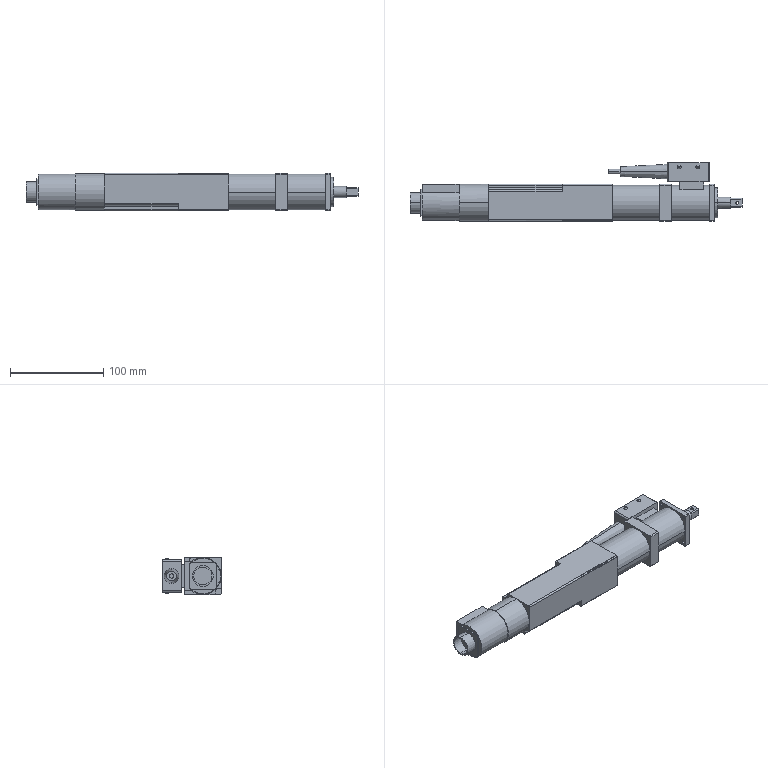Part | STEP file | fNFT-401RM1A-S | 1 solid | 133 faces | box 356.359 x 63.246 x 40.132 mm | volume 479956 mm3 | plane 68 | cylinder 55 | spline 8 | cone 2 | commonest cylinder face diameters 3.15 x15 55.118 x12 3.3 x8 38.1 x5 3.175 x2 4.826 x2